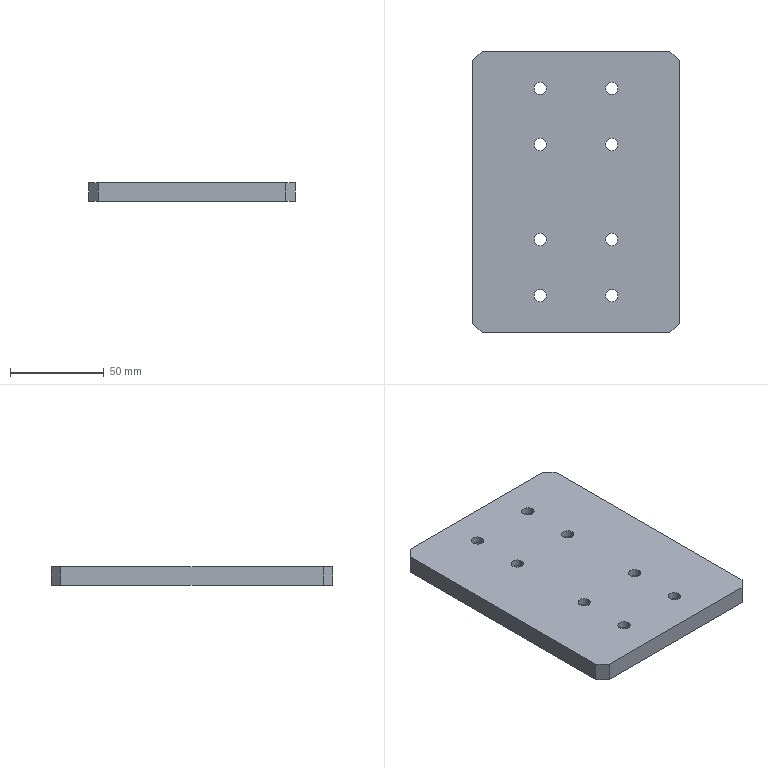Part | SolidWorks | features BaseBody 1 | 1 solid | 50 faces | box 110 x 150 x 10 mm | volume 158649 mm3 | cylinder 32 | plane 18 | commonest cylinder face diameters 6.6 x16 11 x16
STEP:
#1=CARTESIAN_POINT('',(-50.,75.,5.));
#2=VERTEX_POINT('',#1);
#3=CARTESIAN_POINT('',(-55.,70.,5.));
#4=VERTEX_POINT('',#3);
#5=CARTESIAN_POINT('',(-55.,70.,5.));
#6=DIRECTION('',(-0.7071,-0.7071,0.));
#7=VECTOR('',#6,1000.);
#8=LINE('',#5,#7);
#9=EDGE_CURVE('',#2,#4,#8,.T.);
#10=ORIENTED_EDGE('',*,*,#9,.F.);
#11=CARTESIAN_POINT('',(-50.,75.,-5.));
#12=VERTEX_POINT('',#11);
#13=CARTESIAN_POINT('',(-50.,75.,5.));
#14=DIRECTION('',(0.,0.,1.));
#15=VECTOR('',#14,1000.);
#16=LINE('',#13,#15);
#17=EDGE_CURVE('',#12,#2,#16,.T.);
#18=ORIENTED_EDGE('',*,*,#17,.F.);
#19=CARTESIAN_POINT('',(-55.,70.,-5.));
#20=VERTEX_POINT('',#19);
#21=CARTESIAN_POINT('',(-62.5,62.5,-5.));
#22=DIRECTION('',(0.7071,0.7071,0.));
#23=VECTOR('',#22,1000.);
#24=LINE('',#21,#23);
#25=EDGE_CURVE('',#20,#12,#24,.T.);
#26=ORIENTED_EDGE('',*,*,#25,.F.);
#27=CARTESIAN_POINT('',(-55.,70.,5.));
#28=DIRECTION('',(0.,0.,-1.));
#29=VECTOR('',#28,1000.);
#30=LINE('',#27,#29);
#31=EDGE_CURVE('',#4,#20,#30,.T.);
#32=ORIENTED_EDGE('',*,*,#31,.F.);
#33=EDGE_LOOP('',(#10,#18,#26,#32));
#34=FACE_OUTER_BOUND('',#33,.T.);
#35=CARTESIAN_POINT('',(-55.,70.,5.));
#36=DIRECTION('',(0.7071,-0.7071,0.));
#37=DIRECTION('',(0.,0.,-1.));
#38=AXIS2_PLACEMENT_3D('',#35,#36,#37);
#39=PLANE('',#38);
#40=ADVANCED_FACE('',(#34),#39,.F.);
#41=CARTESIAN_POINT('',(55.,70.,5.));
#42=VERTEX_POINT('',#41);
#43=CARTESIAN_POINT('',(50.,75.,5.));
#44=VERTEX_POINT('',#43);
#45=CARTESIAN_POINT('',(50.,75.,5.));
#46=DIRECTION('',(-0.7071,0.7071,0.));
#47=VECTOR('',#46,1000.);
#48=LINE('',#45,#47);
#49=EDGE_CURVE('',#42,#44,#48,.T.);
#50=ORIENTED_EDGE('',*,*,#49,.F.);
#51=CARTESIAN_POINT('',(55.,70.,-5.));
#52=VERTEX_POINT('',#51);
#53=CARTESIAN_POINT('',(55.,70.,5.));
#54=DIRECTION('',(0.,0.,1.));
#55=VECTOR('',#54,1000.);
#56=LINE('',#53,#55);
#57=EDGE_CURVE('',#52,#42,#56,.T.);
#58=ORIENTED_EDGE('',*,*,#57,.F.);
#59=CARTESIAN_POINT('',(50.,75.,-5.));
#60=VERTEX_POINT('',#59);
#61=CARTESIAN_POINT('',(62.5,62.5,-5.));
#62=DIRECTION('',(0.7071,-0.7071,0.));
#63=VECTOR('',#62,1000.);
#64=LINE('',#61,#63);
#65=EDGE_CURVE('',#60,#52,#64,.T.);
#66=ORIENTED_EDGE('',*,*,#65,.F.);
#67=CARTESIAN_POINT('',(50.,75.,5.));
#68=DIRECTION('',(0.,0.,-1.));
#69=VECTOR('',#68,1000.);
#70=LINE('',#67,#69);
#71=EDGE_CURVE('',#44,#60,#70,.T.);
#72=ORIENTED_EDGE('',*,*,#71,.F.);
#73=EDGE_LOOP('',(#50,#58,#66,#72));
#74=FACE_OUTER_BOUND('',#73,.T.);
#75=CARTESIAN_POINT('',(50.,75.,5.));
#76=DIRECTION('',(-0.7071,-0.7071,0.));
#77=DIRECTION('',(-0.7071,0.7071,0.));
#78=AXIS2_PLACEMENT_3D('',#75,#76,#77);
#79=PLANE('',#78);
#80=ADVANCED_FACE('',(#74),#79,.F.);
#81=CARTESIAN_POINT('',(-55.,-70.,5.));
#82=VERTEX_POINT('',#81);
#83=CARTESIAN_POINT('',(-50.,-75.,5.));
#84=VERTEX_POINT('',#83);
#85=CARTESIAN_POINT('',(-50.,-75.,5.));
#86=DIRECTION('',(0.7071,-0.7071,0.));
#87=VECTOR('',#86,1000.);
#88=LINE('',#85,#87);
#89=EDGE_CURVE('',#82,#84,#88,.T.);
#90=ORIENTED_EDGE('',*,*,#89,.F.);
#91=CARTESIAN_POINT('',(-55.,-70.,-5.));
#92=VERTEX_POINT('',#91);
#93=CARTESIAN_POINT('',(-55.,-70.,5.));
#94=DIRECTION('',(0.,0.,1.));
#95=VECTOR('',#94,1000.);
#96=LINE('',#93,#95);
#97=EDGE_CURVE('',#92,#82,#96,.T.);
#98=ORIENTED_EDGE('',*,*,#97,.F.);
#99=CARTESIAN_POINT('',(-50.,-75.,-5.));
#100=VERTEX_POINT('',#99);
#101=CARTESIAN_POINT('',(-62.5,-62.5,-5.));
#102=DIRECTION('',(-0.7071,0.7071,0.));
#103=VECTOR('',#102,1000.);
#104=LINE('',#101,#103);
#105=EDGE_CURVE('',#100,#92,#104,.T.);
#106=ORIENTED_EDGE('',*,*,#105,.F.);
#107=CARTESIAN_POINT('',(-50.,-75.,5.));
#108=DIRECTION('',(0.,0.,-1.));
#109=VECTOR('',#108,1000.);
#110=LINE('',#107,#109);
#111=EDGE_CURVE('',#84,#100,#110,.T.);
#112=ORIENTED_EDGE('',*,*,#111,.F.);
#113=EDGE_LOOP('',(#90,#98,#106,#112));
#114=FACE_OUTER_BOUND('',#113,.T.);
#115=CARTESIAN_POINT('',(-50.,-75.,5.));
#116=DIRECTION('',(0.7071,0.7071,0.));
#117=DIRECTION('',(0.,0.,-1.));
#118=AXIS2_PLACEMENT_3D('',#115,#116,#117);
#119=PLANE('',#118);
#120=ADVANCED_FACE('',(#114),#119,.F.);
#121=CARTESIAN_POINT('',(50.,-75.,5.));
#122=VERTEX_POINT('',#121);
#123=CARTESIAN_POINT('',(55.,-70.,5.));
#124=VERTEX_POINT('',#123);
#125=CARTESIAN_POINT('',(55.,-70.,5.));
#126=DIRECTION('',(0.7071,0.7071,0.));
#127=VECTOR('',#126,1000.);
#128=LINE('',#125,#127);
#129=EDGE_CURVE('',#122,#124,#128,.T.);
#130=ORIENTED_EDGE('',*,*,#129,.F.);
#131=CARTESIAN_POINT('',(50.,-75.,-5.));
#132=VERTEX_POINT('',#131);
#133=CARTESIAN_POINT('',(50.,-75.,5.));
#134=DIRECTION('',(0.,0.,1.));
#135=VECTOR('',#134,1000.);
#136=LINE('',#133,#135);
#137=EDGE_CURVE('',#132,#122,#136,.T.);
#138=ORIENTED_EDGE('',*,*,#137,.F.);
#139=CARTESIAN_POINT('',(55.,-70.,-5.));
#140=VERTEX_POINT('',#139);
#141=CARTESIAN_POINT('',(62.5,-62.5,-5.));
#142=DIRECTION('',(-0.7071,-0.7071,0.));
#143=VECTOR('',#142,1000.);
#144=LINE('',#141,#143);
#145=EDGE_CURVE('',#140,#132,#144,.T.);
#146=ORIENTED_EDGE('',*,*,#145,.F.);
#147=CARTESIAN_POINT('',(55.,-70.,5.));
#148=DIRECTION('',(0.,0.,-1.));
#149=VECTOR('',#148,1000.);
#150=LINE('',#147,#149);
#151=EDGE_CURVE('',#124,#140,#150,.T.);
#152=ORIENTED_EDGE('',*,*,#151,.F.);
#153=EDGE_LOOP('',(#130,#138,#146,#152));
#154=FACE_OUTER_BOUND('',#153,.T.);
#155=CARTESIAN_POINT('',(55.,-70.,5.));
#156=DIRECTION('',(-0.7071,0.7071,0.));
#157=DIRECTION('',(0.,0.,1.));
#158=AXIS2_PLACEMENT_3D('',#155,#156,#157);
#159=PLANE('',#158);
#160=ADVANCED_FACE('',(#154),#159,.F.);
#161=CARTESIAN_POINT('',(-13.5,-55.25,1.4));
#162=VERTEX_POINT('',#161);
#163=CARTESIAN_POINT('',(-13.5,-55.25,-5.));
#164=VERTEX_POINT('',#163);
#165=CARTESIAN_POINT('',(-13.5,-55.25,-5.));
#166=DIRECTION('',(0.,0.,-1.));
#167=VECTOR('',#166,1000.);
#168=LINE('',#165,#167);
#169=EDGE_CURVE('',#162,#164,#168,.T.);
#170=ORIENTED_EDGE('',*,*,#169,.F.);
#171=CARTESIAN_POINT('',(-24.5,-55.25,1.4));
#172=VERTEX_POINT('',#171);
#173=CARTESIAN_POINT('',(-19.,-55.25,1.4));
#174=DIRECTION('',(0.,0.,-1.));
#175=DIRECTION('',(-1.,0.,0.));
#176=AXIS2_PLACEMENT_3D('',#173,#174,#175);
#177=CIRCLE('',#176,5.5);
#178=EDGE_CURVE('',#172,#162,#177,.T.);
#179=ORIENTED_EDGE('',*,*,#178,.F.);
#180=CARTESIAN_POINT('',(-24.5,-55.25,-5.));
#181=VERTEX_POINT('',#180);
#182=CARTESIAN_POINT('',(-24.5,-55.25,-5.));
#183=DIRECTION('',(0.,0.,-1.));
#184=VECTOR('',#183,1000.);
#185=LINE('',#182,#184);
#186=EDGE_CURVE('',#172,#181,#185,.T.);
#187=ORIENTED_EDGE('',*,*,#186,.T.);
#188=CARTESIAN_POINT('',(-19.,-55.25,-5.));
#189=DIRECTION('',(0.,0.,-1.));
#190=DIRECTION('',(-1.,0.,0.));
#191=AXIS2_PLACEMENT_3D('',#188,#189,#190);
#192=CIRCLE('',#191,5.5);
#193=EDGE_CURVE('',#181,#164,#192,.T.);
#194=ORIENTED_EDGE('',*,*,#193,.T.);
#195=EDGE_LOOP('',(#170,#179,#187,#194));
#196=FACE_OUTER_BOUND('',#195,.T.);
#197=CARTESIAN_POINT('',(-19.,-55.25,-5.));
#198=DIRECTION('',(0.,0.,-1.));
#199=DIRECTION('',(-1.,0.,0.));
#200=AXIS2_PLACEMENT_3D('',#197,#198,#199);
#201=CYLINDRICAL_SURFACE('',#200,5.5);
#202=ADVANCED_FACE('',(#196),#201,.F.);
#203=CARTESIAN_POINT('',(-22.3,-55.25,1.4));
#204=VERTEX_POINT('',#203);
#205=CARTESIAN_POINT('',(-15.7,-55.25,1.4));
#206=VERTEX_POINT('',#205);
#207=CARTESIAN_POINT('',(-19.,-55.25,1.4));
#208=DIRECTION('',(0.,0.,-1.));
#209=DIRECTION('',(-1.,0.,0.));
#210=AXIS2_PLACEMENT_3D('',#207,#208,#209);
#211=CIRCLE('',#210,3.3);
#212=EDGE_CURVE('',#204,#206,#211,.T.);
#213=ORIENTED_EDGE('',*,*,#212,.F.);
#214=CARTESIAN_POINT('',(-19.,-55.25,1.4));
#215=DIRECTION('',(0.,0.,-1.));
#216=DIRECTION('',(-1.,0.,0.));
#217=AXIS2_PLACEMENT_3D('',#214,#215,#216);
#218=CIRCLE('',#217,3.3);
#219=EDGE_CURVE('',#206,#204,#218,.T.);
#220=ORIENTED_EDGE('',*,*,#219,.F.);
#221=EDGE_LOOP('',(#213,#220));
#222=FACE_BOUND('',#221,.T.);
#223=ORIENTED_EDGE('',*,*,#178,.T.);
#224=CARTESIAN_POINT('',(-19.,-55.25,1.4));
#225=DIRECTION('',(0.,0.,-1.));
#226=DIRECTION('',(-1.,0.,0.));
#227=AXIS2_PLACEMENT_3D('',#224,#225,#226);
#228=CIRCLE('',#227,5.5);
#229=EDGE_CURVE('',#162,#172,#228,.T.);
#230=ORIENTED_EDGE('',*,*,#229,.T.);
#231=EDGE_LOOP('',(#223,#230));
#232=FACE_OUTER_BOUND('',#231,.T.);
#233=CARTESIAN_POINT('',(-15.7,-55.25,1.4));
#234=DIRECTION('',(0.,0.,1.));
#235=DIRECTION('',(1.,0.,0.));
#236=AXIS2_PLACEMENT_3D('',#233,#234,#235);
#237=PLANE('',#236);
#238=ADVANCED_FACE('',(#222,#232),#237,.F.);
#239=CARTESIAN_POINT('',(-15.7,-55.25,5.));
#240=VERTEX_POINT('',#239);
#241=CARTESIAN_POINT('',(-15.7,-55.25,-5.));
#242=DIRECTION('',(0.,0.,-1.));
#243=VECTOR('',#242,1000.);
#244=LINE('',#241,#243);
#245=EDGE_CURVE('',#240,#206,#244,.T.);
#246=ORIENTED_EDGE('',*,*,#245,.F.);
#247=CARTESIAN_POINT('',(-22.3,-55.25,5.));
#248=VERTEX_POINT('',#247);
#249=CARTESIAN_POINT('',(-19.,-55.25,5.));
#250=DIRECTION('',(0.,0.,-1.));
#251=DIRECTION('',(-1.,0.,0.));
#252=AXIS2_PLACEMENT_3D('',#249,#250,#251);
#253=CIRCLE('',#252,3.3);
#254=EDGE_CURVE('',#248,#240,#253,.T.);
#255=ORIENTED_EDGE('',*,*,#254,.F.);
#256=CARTESIAN_POINT('',(-22.3,-55.25,-5.));
#257=DIRECTION('',(0.,0.,-1.));
#258=VECTOR('',#257,1000.);
#259=LINE('',#256,#258);
#260=EDGE_CURVE('',#248,#204,#259,.T.);
#261=ORIENTED_EDGE('',*,*,#260,.T.);
#262=ORIENTED_EDGE('',*,*,#212,.T.);
#263=EDGE_LOOP('',(#246,#255,#261,#262));
#264=FACE_OUTER_BOUND('',#263,.T.);
#265=CARTESIAN_POINT('',(-19.,-55.25,-5.));
#266=DIRECTION('',(0.,0.,-1.));
#267=DIRECTION('',(-1.,0.,0.));
#268=AXIS2_PLACEMENT_3D('',#265,#266,#267);
#269=CYLINDRICAL_SURFACE('',#268,3.3);
#270=ADVANCED_FACE('',(#264),#269,.F.);
#271=CARTESIAN_POINT('',(-13.5,25.25,1.4));
#272=VERTEX_POINT('',#271);
#273=CARTESIAN_POINT('',(-13.5,25.25,-5.));
#274=VERTEX_POINT('',#273);
#275=CARTESIAN_POINT('',(-13.5,25.25,-5.));
#276=DIRECTION('',(0.,0.,-1.));
#277=VECTOR('',#276,1000.);
#278=LINE('',#275,#277);
#279=EDGE_CURVE('',#272,#274,#278,.T.);
#280=ORIENTED_EDGE('',*,*,#279,.F.);
#281=CARTESIAN_POINT('',(-24.5,25.25,1.4));
#282=VERTEX_POINT('',#281);
#283=CARTESIAN_POINT('',(-19.,25.25,1.4));
#284=DIRECTION('',(0.,0.,-1.));
#285=DIRECTION('',(-1.,0.,0.));
#286=AXIS2_PLACEMENT_3D('',#283,#284,#285);
#287=CIRCLE('',#286,5.5);
#288=EDGE_CURVE('',#282,#272,#287,.T.);
#289=ORIENTED_EDGE('',*,*,#288,.F.);
#290=CARTESIAN_POINT('',(-24.5,25.25,-5.));
#291=VERTEX_POINT('',#290);
#292=CARTESIAN_POINT('',(-24.5,25.25,-5.));
#293=DIRECTION('',(0.,0.,-1.));
#294=VECTOR('',#293,1000.);
#295=LINE('',#292,#294);
#296=EDGE_CURVE('',#282,#291,#295,.T.);
#297=ORIENTED_EDGE('',*,*,#296,.T.);
#298=CARTESIAN_POINT('',(-19.,25.25,-5.));
#299=DIRECTION('',(0.,0.,-1.));
#300=DIRECTION('',(-1.,0.,0.));
#301=AXIS2_PLACEMENT_3D('',#298,#299,#300);
#302=CIRCLE('',#301,5.5);
#303=EDGE_CURVE('',#291,#274,#302,.T.);
#304=ORIENTED_EDGE('',*,*,#303,.T.);
#305=EDGE_LOOP('',(#280,#289,#297,#304));
#306=FACE_OUTER_BOUND('',#305,.T.);
#307=CARTESIAN_POINT('',(-19.,25.25,-5.));
#308=DIRECTION('',(0.,0.,-1.));
#309=DIRECTION('',(-1.,0.,0.));
#310=AXIS2_PLACEMENT_3D('',#307,#308,#309);
#311=CYLINDRICAL_SURFACE('',#310,5.5);
#312=ADVANCED_FACE('',(#306),#311,.F.);
#313=CARTESIAN_POINT('',(-22.3,25.25,1.4));
#314=VERTEX_POINT('',#313);
#315=CARTESIAN_POINT('',(-15.7,25.25,1.4));
#316=VERTEX_POINT('',#315);
#317=CARTESIAN_POINT('',(-19.,25.25,1.4));
#318=DIRECTION('',(0.,0.,-1.));
#319=DIRECTION('',(-1.,0.,0.));
#320=AXIS2_PLACEMENT_3D('',#317,#318,#319);
#321=CIRCLE('',#320,3.3);
#322=EDGE_CURVE('',#314,#316,#321,.T.);
#323=ORIENTED_EDGE('',*,*,#322,.F.);
#324=CARTESIAN_POINT('',(-19.,25.25,1.4));
#325=DIRECTION('',(0.,0.,-1.));
#326=DIRECTION('',(-1.,0.,0.));
#327=AXIS2_PLACEMENT_3D('',#324,#325,#326);
#328=CIRCLE('',#327,3.3);
#329=EDGE_CURVE('',#316,#314,#328,.T.);
#330=ORIENTED_EDGE('',*,*,#329,.F.);
#331=EDGE_LOOP('',(#323,#330));
#332=FACE_BOUND('',#331,.T.);
#333=ORIENTED_EDGE('',*,*,#288,.T.);
#334=CARTESIAN_POINT('',(-19.,25.25,1.4));
#335=DIRECTION('',(0.,0.,-1.));
#336=DIRECTION('',(-1.,0.,0.));
#337=AXIS2_PLACEMENT_3D('',#334,#335,#336);
#338=CIRCLE('',#337,5.5);
#339=EDGE_CURVE('',#272,#282,#338,.T.);
#340=ORIENTED_EDGE('',*,*,#339,.T.);
#341=EDGE_LOOP('',(#333,#340));
#342=FACE_OUTER_BOUND('',#341,.T.);
#343=CARTESIAN_POINT('',(-15.7,25.25,1.4));
#344=DIRECTION('',(0.,0.,1.));
#345=DIRECTION('',(1.,0.,0.));
#346=AXIS2_PLACEMENT_3D('',#343,#344,#345);
#347=PLANE('',#346);
#348=ADVANCED_FACE('',(#332,#342),#347,.F.);
#349=CARTESIAN_POINT('',(-15.7,25.25,5.));
#350=VERTEX_POINT('',#349);
#351=CARTESIAN_POINT('',(-15.7,25.25,-5.));
#352=DIRECTION('',(0.,0.,-1.));
#353=VECTOR('',#352,1000.);
#354=LINE('',#351,#353);
#355=EDGE_CURVE('',#350,#316,#354,.T.);
#356=ORIENTED_EDGE('',*,*,#355,.F.);
#357=CARTESIAN_POINT('',(-22.3,25.25,5.));
#358=VERTEX_POINT('',#357);
#359=CARTESIAN_POINT('',(-19.,25.25,5.));
#360=DIRECTION('',(0.,0.,-1.));
#361=DIRECTION('',(-1.,0.,0.));
#362=AXIS2_PLACEMENT_3D('',#359,#360,#361);
#363=CIRCLE('',#362,3.3);
#364=EDGE_CURVE('',#358,#350,#363,.T.);
#365=ORIENTED_EDGE('',*,*,#364,.F.);
#366=CARTESIAN_POINT('',(-22.3,25.25,-5.));
#367=DIRECTION('',(0.,0.,-1.));
#368=VECTOR('',#367,1000.);
#369=LINE('',#366,#368);
#370=EDGE_CURVE('',#358,#314,#369,.T.);
#371=ORIENTED_EDGE('',*,*,#370,.T.);
#372=ORIENTED_EDGE('',*,*,#322,.T.);
#373=EDGE_LOOP('',(#356,#365,#371,#372));
#374=FACE_OUTER_BOUND('',#373,.T.);
#375=CARTESIAN_POINT('',(-19.,25.25,-5.));
#376=DIRECTION('',(0.,0.,-1.));
#377=DIRECTION('',(-1.,0.,0.));
#378=AXIS2_PLACEMENT_3D('',#375,#376,#377);
#379=CYLINDRICAL_SURFACE('',#378,3.3);
#380=ADVANCED_FACE('',(#374),#379,.F.);
#381=CARTESIAN_POINT('',(-13.5,55.25,1.4));
#382=VERTEX_POINT('',#381);
#383=CARTESIAN_POINT('',(-13.5,55.25,-5.));
#384=VERTEX_POINT('',#383);
#385=CARTESIAN_POINT('',(-13.5,55.25,-5.));
#386=DIRECTION('',(0.,0.,-1.));
#387=VECTOR('',#386,1000.);
#388=LINE('',#385,#387);
#389=EDGE_CURVE('',#382,#384,#388,.T.);
#390=ORIENTED_EDGE('',*,*,#389,.F.);
#391=CARTESIAN_POINT('',(-24.5,55.25,1.4));
#392=VERTEX_POINT('',#391);
#393=CARTESIAN_POINT('',(-19.,55.25,1.4));
#394=DIRECTION('',(0.,0.,-1.));
#395=DIRECTION('',(-1.,0.,0.));
#396=AXIS2_PLACEMENT_3D('',#393,#394,#395);
#397=CIRCLE('',#396,5.5);
#398=EDGE_CURVE('',#392,#382,#397,.T.);
#399=ORIENTED_EDGE('',*,*,#398,.F.);
#400=CARTESIAN_POINT('',(-24.5,55.25,-5.));
#401=VERTEX_POINT('',#400);
#402=CARTESIAN_POINT('',(-24.5,55.25,-5.));
#403=DIRECTION('',(0.,0.,-1.));
#404=VECTOR('',#403,1000.);
#405=LINE('',#402,#404);
#406=EDGE_CURVE('',#392,#401,#405,.T.);
#407=ORIENTED_EDGE('',*,*,#406,.T.);
#408=CARTESIAN_POINT('',(-19.,55.25,-5.));
#409=DIRECTION('',(0.,0.,-1.));
#410=DIRECTION('',(-1.,0.,0.));
#411=AXIS2_PLACEMENT_3D('',#408,#409,#410);
#412=CIRCLE('',#411,5.5);
#413=EDGE_CURVE('',#401,#384,#412,.T.);
#414=ORIENTED_EDGE('',*,*,#413,.T.);
#415=EDGE_LOOP('',(#390,#399,#407,#414));
#416=FACE_OUTER_BOUND('',#415,.T.);
#417=CARTESIAN_POINT('',(-19.,55.25,-5.));
#418=DIRECTION('',(0.,0.,-1.));
#419=DIRECTION('',(-1.,0.,0.));
#420=AXIS2_PLACEMENT_3D('',#417,#418,#419);
#421=CYLINDRICAL_SURFACE('',#420,5.5);
#422=ADVANCED_FACE('',(#416),#421,.F.);
#423=CARTESIAN_POINT('',(-22.3,55.25,1.4));
#424=VERTEX_POINT('',#423);
#425=CARTESIAN_POINT('',(-15.7,55.25,1.4));
#426=VERTEX_POINT('',#425);
#427=CARTESIAN_POINT('',(-19.,55.25,1.4));
#428=DIRECTION('',(0.,0.,-1.));
#429=DIRECTION('',(-1.,0.,0.));
#430=AXIS2_PLACEMENT_3D('',#427,#428,#429);
#431=CIRCLE('',#430,3.3);
#432=EDGE_CURVE('',#424,#426,#431,.T.);
#433=ORIENTED_EDGE('',*,*,#432,.F.);
#434=CARTESIAN_POINT('',(-19.,55.25,1.4));
#435=DIRECTION('',(0.,0.,-1.));
#436=DIRECTION('',(-1.,0.,0.));
#437=AXIS2_PLACEMENT_3D('',#434,#435,#436);
#438=CIRCLE('',#437,3.3);
#439=EDGE_CURVE('',#426,#424,#438,.T.);
#440=ORIENTED_EDGE('',*,*,#439,.F.);
#441=EDGE_LOOP('',(#433,#440));
#442=FACE_BOUND('',#441,.T.);
#443=ORIENTED_EDGE('',*,*,#398,.T.);
#444=CARTESIAN_POINT('',(-19.,55.25,1.4));
#445=DIRECTION('',(0.,0.,-1.));
#446=DIRECTION('',(-1.,0.,0.));
#447=AXIS2_PLACEMENT_3D('',#444,#445,#446);
#448=CIRCLE('',#447,5.5);
#449=EDGE_CURVE('',#382,#392,#448,.T.);
#450=ORIENTED_EDGE('',*,*,#449,.T.);
#451=EDGE_LOOP('',(#443,#450));
#452=FACE_OUTER_BOUND('',#451,.T.);
#453=CARTESIAN_POINT('',(-15.7,55.25,1.4));
#454=DIRECTION('',(0.,0.,1.));
#455=DIRECTION('',(1.,0.,0.));
#456=AXIS2_PLACEMENT_3D('',#453,#454,#455);
#457=PLANE('',#456);
#458=ADVANCED_FACE('',(#442,#452),#457,.F.);
#459=CARTESIAN_POINT('',(-15.7,55.25,5.));
#460=VERTEX_POINT('',#459);
#461=CARTESIAN_POINT('',(-15.7,55.25,-5.));
#462=DIRECTION('',(0.,0.,-1.));
#463=VECTOR('',#462,1000.);
#464=LINE('',#461,#463);
#465=EDGE_CURVE('',#460,#426,#464,.T.);
#466=ORIENTED_EDGE('',*,*,#465,.F.);
#467=CARTESIAN_POINT('',(-22.3,55.25,5.));
#468=VERTEX_POINT('',#467);
#469=CARTESIAN_POINT('',(-19.,55.25,5.));
#470=DIRECTION('',(0.,0.,-1.));
#471=DIRECTION('',(-1.,0.,0.));
#472=AXIS2_PLACEMENT_3D('',#469,#470,#471);
#473=CIRCLE('',#472,3.3);
#474=EDGE_CURVE('',#468,#460,#473,.T.);
#475=ORIENTED_EDGE('',*,*,#474,.F.);
#476=CARTESIAN_POINT('',(-22.3,55.25,-5.));
#477=DIRECTION('',(0.,0.,-1.));
#478=VECTOR('',#477,1000.);
#479=LINE('',#476,#478);
#480=EDGE_CURVE('',#468,#424,#479,.T.);
#481=ORIENTED_EDGE('',*,*,#480,.T.);
#482=ORIENTED_EDGE('',*,*,#432,.T.);
#483=EDGE_LOOP('',(#466,#475,#481,#482));
#484=FACE_OUTER_BOUND('',#483,.T.);
#485=CARTESIAN_POINT('',(-19.,55.25,-5.));
#486=DIRECTION('',(0.,0.,-1.));
#487=DIRECTION('',(-1.,0.,0.));
#488=AXIS2_PLACEMENT_3D('',#485,#486,#487);
#489=CYLINDRICAL_SURFACE('',#488,3.3);
#490=ADVANCED_FACE('',(#484),#489,.F.);
#491=CARTESIAN_POINT('',(-13.5,-25.25,1.4));
#492=VERTEX_POINT('',#491);
#493=CARTESIAN_POINT('',(-13.5,-25.25,-5.));
#494=VERTEX_POINT('',#493);
#495=CARTESIAN_POINT('',(-13.5,-25.25,-5.));
#496=DIRECTION('',(0.,0.,-1.));
#497=VECTOR('',#496,1000.);
#498=LINE('',#495,#497);
#499=EDGE_CURVE('',#492,#494,#498,.T.);
#500=ORIENTED_EDGE('',*,*,#499,.F.);
#501=CARTESIAN_POINT('',(-24.5,-25.25,1.4));
#502=VERTEX_POINT('',#501);
#503=CARTESIAN_POINT('',(-19.,-25.25,1.4));
#504=DIRECTION('',(0.,0.,-1.));
#505=DIRECTION('',(-1.,0.,0.));
#506=AXIS2_PLACEMENT_3D('',#503,#504,#505);
#507=CIRCLE('',#506,5.5);
#508=EDGE_CURVE('',#502,#492,#507,.T.);
#509=ORIENTED_EDGE('',*,*,#508,.F.);
#510=CARTESIAN_POINT('',(-24.5,-25.25,-5.));
#511=VERTEX_POINT('',#510);
#512=CARTESIAN_POINT('',(-24.5,-25.25,-5.));
#513=DIRECTION('',(0.,0.,-1.));
#514=VECTOR('',#513,1000.);
#515=LINE('',#512,#514);
#516=EDGE_CURVE('',#502,#511,#515,.T.);
#517=ORIENTED_EDGE('',*,*,#516,.T.);
#518=CARTESIAN_POINT('',(-19.,-25.25,-5.));
#519=DIRECTION('',(0.,0.,-1.));
#520=DIRECTION('',(-1.,0.,0.));
#521=AXIS2_PLACEMENT_3D('',#518,#519,#520);
#522=CIRCLE('',#521,5.5);
#523=EDGE_CURVE('',#511,#494,#522,.T.);
#524=ORIENTED_EDGE('',*,*,#523,.T.);
#525=EDGE_LOOP('',(#500,#509,#517,#524));
#526=FACE_OUTER_BOUND('',#525,.T.);
#527=CARTESIAN_POINT('',(-19.,-25.25,-5.));
#528=DIRECTION('',(0.,0.,-1.));
#529=DIRECTION('',(-1.,0.,0.));
#530=AXIS2_PLACEMENT_3D('',#527,#528,#529);
#531=CYLINDRICAL_SURFACE('',#530,5.5);
#532=ADVANCED_FACE('',(#526),#531,.F.);
#533=CARTESIAN_POINT('',(-22.3,-25.25,1.4));
#534=VERTEX_POINT('',#533);
#535=CARTESIAN_POINT('',(-15.7,-25.25,1.4));
#536=VERTEX_POINT('',#535);
#537=CARTESIAN_POINT('',(-19.,-25.25,1.4));
#538=DIRECTION('',(0.,0.,-1.));
#539=DIRECTION('',(-1.,0.,0.));
#540=AXIS2_PLACEMENT_3D('',#537,#538,#539);
#541=CIRCLE('',#540,3.3);
#542=EDGE_CURVE('',#534,#536,#541,.T.);
#543=ORIENTED_EDGE('',*,*,#542,.F.);
#544=CARTESIAN_POINT('',(-19.,-25.25,1.4));
#545=DIRECTION('',(0.,0.,-1.));
#546=DIRECTION('',(-1.,0.,0.));
#547=AXIS2_PLACEMENT_3D('',#544,#545,#546);
#548=CIRCLE('',#547,3.3);
#549=EDGE_CURVE('',#536,#534,#548,.T.);
#550=ORIENTED_EDGE('',*,*,#549,.F.);
#551=EDGE_LOOP('',(#543,#550));
#552=FACE_BOUND('',#551,.T.);
#553=ORIENTED_EDGE('',*,*,#508,.T.);
#554=CARTESIAN_POINT('',(-19.,-25.25,1.4));
#555=DIRECTION('',(0.,0.,-1.));
#556=DIRECTION('',(-1.,0.,0.));
#557=AXIS2_PLACEMENT_3D('',#554,#555,#556);
#558=CIRCLE('',#557,5.5);
#559=EDGE_CURVE('',#492,#502,#558,.T.);
#560=ORIENTED_EDGE('',*,*,#559,.T.);
#561=EDGE_LOOP('',(#553,#560));
#562=FACE_OUTER_BOUND('',#561,.T.);
#563=CARTESIAN_POINT('',(-15.7,-25.25,1.4));
#564=DIRECTION('',(0.,0.,1.));
#565=DIRECTION('',(1.,0.,0.));
#566=AXIS2_PLACEMENT_3D('',#563,#564,#565);
#567=PLANE('',#566);
#568=ADVANCED_FACE('',(#552,#562),#567,.F.);
#569=CARTESIAN_POINT('',(-15.7,-25.25,5.));
#570=VERTEX_POINT('',#569);
#571=CARTESIAN_POINT('',(-15.7,-25.25,-5.));
#572=DIRECTION('',(0.,0.,-1.));
#573=VECTOR('',#572,1000.);
#574=LINE('',#571,#573);
#575=EDGE_CURVE('',#570,#536,#574,.T.);
#576=ORIENTED_EDGE('',*,*,#575,.F.);
#577=CARTESIAN_POINT('',(-22.3,-25.25,5.));
#578=VERTEX_POINT('',#577);
#579=CARTESIAN_POINT('',(-19.,-25.25,5.));
#580=DIRECTION('',(0.,0.,-1.));
#581=DIRECTION('',(-1.,0.,0.));
#582=AXIS2_PLACEMENT_3D('',#579,#580,#581);
#583=CIRCLE('',#582,3.3);
#584=EDGE_CURVE('',#578,#570,#583,.T.);
#585=ORIENTED_EDGE('',*,*,#584,.F.);
#586=CARTESIAN_POINT('',(-22.3,-25.25,-5.));
#587=DIRECTION('',(0.,0.,-1.));
#588=VECTOR('',#587,1000.);
#589=LINE('',#586,#588);
#590=EDGE_CURVE('',#578,#534,#589,.T.);
#591=ORIENTED_EDGE('',*,*,#590,.T.);
#592=ORIENTED_EDGE('',*,*,#542,.T.);
#593=EDGE_LOOP('',(#576,#585,#591,#592));
#594=FACE_OUTER_BOUND('',#593,.T.);
#595=CARTESIAN_POINT('',(-19.,-25.25,-5.));
#596=DIRECTION('',(0.,0.,-1.));
#597=DIRECTION('',(-1.,0.,0.));
#598=AXIS2_PLACEMENT_3D('',#595,#596,#597);
#599=CYLINDRICAL_SURFACE('',#598,3.3);
#600=ADVANCED_FACE('',(#594),#599,.F.);
#601=CARTESIAN_POINT('',(24.5,-55.25,1.4));
#602=VERTEX_POINT('',#601);
#603=CARTESIAN_POINT('',(24.5,-55.25,-5.));
#604=VERTEX_POINT('',#603);
#605=CARTESIAN_POINT('',(24.5,-55.25,-5.));
#606=DIRECTION('',(0.,0.,-1.));
#607=VECTOR('',#606,1000.);
#608=LINE('',#605,#607);
#609=EDGE_CURVE('',#602,#604,#608,.T.);
#610=ORIENTED_EDGE('',*,*,#609,.F.);
#611=CARTESIAN_POINT('',(13.5,-55.25,1.4));
#612=VERTEX_POINT('',#611);
#613=CARTESIAN_POINT('',(19.,-55.25,1.4));
#614=DIRECTION('',(0.,0.,-1.));
#615=DIRECTION('',(-1.,0.,0.));
#616=AXIS2_PLACEMENT_3D('',#613,#614,#615);
#617=CIRCLE('',#616,5.5);
#618=EDGE_CURVE('',#612,#602,#617,.T.);
#619=ORIENTED_EDGE('',*,*,#618,.F.);
#620=CARTESIAN_POINT('',(13.5,-55.25,-5.));
#621=VERTEX_POINT('',#620);
#622=CARTESIAN_POINT('',(13.5,-55.25,-5.));
#623=DIRECTION('',(0.,0.,-1.));
#624=VECTOR('',#623,1000.);
#625=LINE('',#622,#624);
#626=EDGE_CURVE('',#612,#621,#625,.T.);
#627=ORIENTED_EDGE('',*,*,#626,.T.);
#628=CARTESIAN_POINT('',(19.,-55.25,-5.));
#629=DIRECTION('',(0.,0.,-1.));
#630=DIRECTION('',(-1.,0.,0.));
#631=AXIS2_PLACEMENT_3D('',#628,#629,#630);
#632=CIRCLE('',#631,5.5);
#633=EDGE_CURVE('',#621,#604,#632,.T.);
#634=ORIENTED_EDGE('',*,*,#633,.T.);
#635=EDGE_LOOP('',(#610,#619,#627,#634));
#636=FACE_OUTER_BOUND('',#635,.T.);
#637=CARTESIAN_POINT('',(19.,-55.25,-5.));
#638=DIRECTION('',(0.,0.,-1.));
#639=DIRECTION('',(-1.,0.,0.));
#640=AXIS2_PLACEMENT_3D('',#637,#638,#639);
#641=CYLINDRICAL_SURFACE('',#640,5.5);
#642=ADVANCED_FACE('',(#636),#641,.F.);
#643=CARTESIAN_POINT('',(15.7,-55.25,1.4));
#644=VERTEX_POINT('',#643);
#645=CARTESIAN_POINT('',(22.3,-55.25,1.4));
#646=VERTEX_POINT('',#645);
#647=CARTESIAN_POINT('',(19.,-55.25,1.4));
#648=DIRECTION('',(0.,0.,-1.));
#649=DIRECTION('',(-1.,0.,0.));
#650=AXIS2_PLACEMENT_3D('',#647,#648,#649);
#651=CIRCLE('',#650,3.3);
#652=EDGE_CURVE('',#644,#646,#651,.T.);
#653=ORIENTED_EDGE('',*,*,#652,.F.);
#654=CARTESIAN_POINT('',(19.,-55.25,1.4));
#655=DIRECTION('',(0.,0.,-1.));
#656=DIRECTION('',(-1.,0.,0.));
#657=AXIS2_PLACEMENT_3D('',#654,#655,#656);
#658=CIRCLE('',#657,3.3);
#659=EDGE_CURVE('',#646,#644,#658,.T.);
#660=ORIENTED_EDGE('',*,*,#659,.F.);
#661=EDGE_LOOP('',(#653,#660));
#662=FACE_BOUND('',#661,.T.);
#663=ORIENTED_EDGE('',*,*,#618,.T.);
#664=CARTESIAN_POINT('',(19.,-55.25,1.4));
#665=DIRECTION('',(0.,0.,-1.));
#666=DIRECTION('',(-1.,0.,0.));
#667=AXIS2_PLACEMENT_3D('',#664,#665,#666);
#668=CIRCLE('',#667,5.5);
#669=EDGE_CURVE('',#602,#612,#668,.T.);
#670=ORIENTED_EDGE('',*,*,#669,.T.);
#671=EDGE_LOOP('',(#663,#670));
#672=FACE_OUTER_BOUND('',#671,.T.);
#673=CARTESIAN_POINT('',(22.3,-55.25,1.4));
#674=DIRECTION('',(0.,0.,1.));
#675=DIRECTION('',(1.,0.,0.));
#676=AXIS2_PLACEMENT_3D('',#673,#674,#675);
#677=PLANE('',#676);
#678=ADVANCED_FACE('',(#662,#672),#677,.F.);
#679=CARTESIAN_POINT('',(22.3,-55.25,5.));
#680=VERTEX_POINT('',#679);
#681=CARTESIAN_POINT('',(22.3,-55.25,-5.));
#682=DIRECTION('',(0.,0.,-1.));
#683=VECTOR('',#682,1000.);
#684=LINE('',#681,#683);
#685=EDGE_CURVE('',#680,#646,#684,.T.);
#686=ORIENTED_EDGE('',*,*,#685,.F.);
#687=CARTESIAN_POINT('',(15.7,-55.25,5.));
#688=VERTEX_POINT('',#687);
#689=CARTESIAN_POINT('',(19.,-55.25,5.));
#690=DIRECTION('',(0.,0.,-1.));
#691=DIRECTION('',(-1.,0.,0.));
#692=AXIS2_PLACEMENT_3D('',#689,#690,#691);
#693=CIRCLE('',#692,3.3);
#694=EDGE_CURVE('',#688,#680,#693,.T.);
#695=ORIENTED_EDGE('',*,*,#694,.F.);
#696=CARTESIAN_POINT('',(15.7,-55.25,-5.));
#697=DIRECTION('',(0.,0.,-1.));
#698=VECTOR('',#697,1000.);
#699=LINE('',#696,#698);
#700=EDGE_CURVE('',#688,#644,#699,.T.);
#701=ORIENTED_EDGE('',*,*,#700,.T.);
#702=ORIENTED_EDGE('',*,*,#652,.T.);
#703=EDGE_LOOP('',(#686,#695,#701,#702));
#704=FACE_OUTER_BOUND('',#703,.T.);
#705=CARTESIAN_POINT('',(19.,-55.25,-5.));
#706=DIRECTION('',(0.,0.,-1.));
#707=DIRECTION('',(-1.,0.,0.));
#708=AXIS2_PLACEMENT_3D('',#705,#706,#707);
#709=CYLINDRICAL_SURFACE('',#708,3.3);
#710=ADVANCED_FACE('',(#704),#709,.F.);
#711=CARTESIAN_POINT('',(24.5,-25.25,1.4));
#712=VERTEX_POINT('',#711);
#713=CARTESIAN_POINT('',(24.5,-25.25,-5.));
#714=VERTEX_POINT('',#713);
#715=CARTESIAN_POINT('',(24.5,-25.25,-5.));
#716=DIRECTION('',(0.,0.,-1.));
#717=VECTOR('',#716,1000.);
#718=LINE('',#715,#717);
#719=EDGE_CURVE('',#712,#714,#718,.T.);
#720=ORIENTED_EDGE('',*,*,#719,.F.);
#721=CARTESIAN_POINT('',(13.5,-25.25,1.4));
#722=VERTEX_POINT('',#721);
#723=CARTESIAN_POINT('',(19.,-25.25,1.4));
#724=DIRECTION('',(0.,0.,-1.));
#725=DIRECTION('',(-1.,0.,0.));
#726=AXIS2_PLACEMENT_3D('',#723,#724,#725);
#727=CIRCLE('',#726,5.5);
#728=EDGE_CURVE('',#722,#712,#727,.T.);
#729=ORIENTED_EDGE('',*,*,#728,.F.);
#730=CARTESIAN_POINT('',(13.5,-25.25,-5.));
#731=VERTEX_POINT('',#730);
#732=CARTESIAN_POINT('',(13.5,-25.25,-5.));
#733=DIRECTION('',(0.,0.,-1.));
#734=VECTOR('',#733,1000.);
#735=LINE('',#732,#734);
#736=EDGE_CURVE('',#722,#731,#735,.T.);
#737=ORIENTED_EDGE('',*,*,#736,.T.);
#738=CARTESIAN_POINT('',(19.,-25.25,-5.));
#739=DIRECTION('',(0.,0.,-1.));
#740=DIRECTION('',(-1.,0.,0.));
#741=AXIS2_PLACEMENT_3D('',#738,#739,#740);
#742=CIRCLE('',#741,5.5);
#743=EDGE_CURVE('',#731,#714,#742,.T.);
#744=ORIENTED_EDGE('',*,*,#743,.T.);
#745=EDGE_LOOP('',(#720,#729,#737,#744));
#746=FACE_OUTER_BOUND('',#745,.T.);
#747=CARTESIAN_POINT('',(19.,-25.25,-5.));
#748=DIRECTION('',(0.,0.,-1.));
#749=DIRECTION('',(-1.,0.,0.));
#750=AXIS2_PLACEMENT_3D('',#747,#748,#749);
#751=CYLINDRICAL_SURFACE('',#750,5.5);
#752=ADVANCED_FACE('',(#746),#751,.F.);
#753=CARTESIAN_POINT('',(15.7,-25.25,1.4));
#754=VERTEX_POINT('',#753);
#755=CARTESIAN_POINT('',(22.3,-25.25,1.4));
#756=VERTEX_POINT('',#755);
#757=CARTESIAN_POINT('',(19.,-25.25,1.4));
#758=DIRECTION('',(0.,0.,-1.));
#759=DIRECTION('',(-1.,0.,0.));
#760=AXIS2_PLACEMENT_3D('',#757,#758,#759);
#761=CIRCLE('',#760,3.3);
#762=EDGE_CURVE('',#754,#756,#761,.T.);
#763=ORIENTED_EDGE('',*,*,#762,.F.);
#764=CARTESIAN_POINT('',(19.,-25.25,1.4));
#765=DIRECTION('',(0.,0.,-1.));
#766=DIRECTION('',(-1.,0.,0.));
#767=AXIS2_PLACEMENT_3D('',#764,#765,#766);
#768=CIRCLE('',#767,3.3);
#769=EDGE_CURVE('',#756,#754,#768,.T.);
#770=ORIENTED_EDGE('',*,*,#769,.F.);
#771=EDGE_LOOP('',(#763,#770));
#772=FACE_BOUND('',#771,.T.);
#773=ORIENTED_EDGE('',*,*,#728,.T.);
#774=CARTESIAN_POINT('',(19.,-25.25,1.4));
#775=DIRECTION('',(0.,0.,-1.));
#776=DIRECTION('',(-1.,0.,0.));
#777=AXIS2_PLACEMENT_3D('',#774,#775,#776);
#778=CIRCLE('',#777,5.5);
#779=EDGE_CURVE('',#712,#722,#778,.T.);
#780=ORIENTED_EDGE('',*,*,#779,.T.);
#781=EDGE_LOOP('',(#773,#780));
#782=FACE_OUTER_BOUND('',#781,.T.);
#783=CARTESIAN_POINT('',(22.3,-25.25,1.4));
#784=DIRECTION('',(0.,0.,1.));
#785=DIRECTION('',(1.,0.,0.));
#786=AXIS2_PLACEMENT_3D('',#783,#784,#785);
#787=PLANE('',#786);
#788=ADVANCED_FACE('',(#772,#782),#787,.F.);
#789=CARTESIAN_POINT('',(22.3,-25.25,5.));
#790=VERTEX_POINT('',#789);
#791=CARTESIAN_POINT('',(22.3,-25.25,-5.));
#792=DIRECTION('',(0.,0.,-1.));
#793=VECTOR('',#792,1000.);
#794=LINE('',#791,#793);
#795=EDGE_CURVE('',#790,#756,#794,.T.);
#796=ORIENTED_EDGE('',*,*,#795,.F.);
#797=CARTESIAN_POINT('',(15.7,-25.25,5.));
#798=VERTEX_POINT('',#797);
#799=CARTESIAN_POINT('',(19.,-25.25,5.));
#800=DIRECTION('',(0.,0.,-1.));
#801=DIRECTION('',(-1.,0.,0.));
#802=AXIS2_PLACEMENT_3D('',#799,#800,#801);
#803=CIRCLE('',#802,3.3);
#804=EDGE_CURVE('',#798,#790,#803,.T.);
#805=ORIENTED_EDGE('',*,*,#804,.F.);
#806=CARTESIAN_POINT('',(15.7,-25.25,-5.));
#807=DIRECTION('',(0.,0.,-1.));
#808=VECTOR('',#807,1000.);
#809=LINE('',#806,#808);
#810=EDGE_CURVE('',#798,#754,#809,.T.);
#811=ORIENTED_EDGE('',*,*,#810,.T.);
#812=ORIENTED_EDGE('',*,*,#762,.T.);
#813=EDGE_LOOP('',(#796,#805,#811,#812));
#814=FACE_OUTER_BOUND('',#813,.T.);
#815=CARTESIAN_POINT('',(19.,-25.25,-5.));
#816=DIRECTION('',(0.,0.,-1.));
#817=DIRECTION('',(-1.,0.,0.));
#818=AXIS2_PLACEMENT_3D('',#815,#816,#817);
#819=CYLINDRICAL_SURFACE('',#818,3.3);
#820=ADVANCED_FACE('',(#814),#819,.F.);
#821=CARTESIAN_POINT('',(24.5,25.25,1.4));
#822=VERTEX_POINT('',#821);
#823=CARTESIAN_POINT('',(24.5,25.25,-5.));
#824=VERTEX_POINT('',#823);
#825=CARTESIAN_POINT('',(24.5,25.25,-5.));
#826=DIRECTION('',(0.,0.,-1.));
#827=VECTOR('',#826,1000.);
#828=LINE('',#825,#827);
#829=EDGE_CURVE('',#822,#824,#828,.T.);
#830=ORIENTED_EDGE('',*,*,#829,.F.);
#831=CARTESIAN_POINT('',(13.5,25.25,1.4));
#832=VERTEX_POINT('',#831);
#833=CARTESIAN_POINT('',(19.,25.25,1.4));
#834=DIRECTION('',(0.,0.,-1.));
#835=DIRECTION('',(-1.,0.,0.));
#836=AXIS2_PLACEMENT_3D('',#833,#834,#835);
#837=CIRCLE('',#836,5.5);
#838=EDGE_CURVE('',#832,#822,#837,.T.);
#839=ORIENTED_EDGE('',*,*,#838,.F.);
#840=CARTESIAN_POINT('',(13.5,25.25,-5.));
#841=VERTEX_POINT('',#840);
#842=CARTESIAN_POINT('',(13.5,25.25,-5.));
#843=DIRECTION('',(0.,0.,-1.));
#844=VECTOR('',#843,1000.);
#845=LINE('',#842,#844);
#846=EDGE_CURVE('',#832,#841,#845,.T.);
#847=ORIENTED_EDGE('',*,*,#846,.T.);
#848=CARTESIAN_POINT('',(19.,25.25,-5.));
#849=DIRECTION('',(0.,0.,-1.));
#850=DIRECTION('',(-1.,0.,0.));
#851=AXIS2_PLACEMENT_3D('',#848,#849,#850);
#852=CIRCLE('',#851,5.5);
#853=EDGE_CURVE('',#841,#824,#852,.T.);
#854=ORIENTED_EDGE('',*,*,#853,.T.);
#855=EDGE_LOOP('',(#830,#839,#847,#854));
#856=FACE_OUTER_BOUND('',#855,.T.);
#857=CARTESIAN_POINT('',(19.,25.25,-5.));
#858=DIRECTION('',(0.,0.,-1.));
#859=DIRECTION('',(-1.,0.,0.));
#860=AXIS2_PLACEMENT_3D('',#857,#858,#859);
#861=CYLINDRICAL_SURFACE('',#860,5.5);
#862=ADVANCED_FACE('',(#856),#861,.F.);
#863=CARTESIAN_POINT('',(15.7,25.25,1.4));
#864=VERTEX_POINT('',#863);
#865=CARTESIAN_POINT('',(22.3,25.25,1.4));
#866=VERTEX_POINT('',#865);
#867=CARTESIAN_POINT('',(19.,25.25,1.4));
#868=DIRECTION('',(0.,0.,-1.));
#869=DIRECTION('',(-1.,0.,0.));
#870=AXIS2_PLACEMENT_3D('',#867,#868,#869);
#871=CIRCLE('',#870,3.3);
#872=EDGE_CURVE('',#864,#866,#871,.T.);
#873=ORIENTED_EDGE('',*,*,#872,.F.);
#874=CARTESIAN_POINT('',(19.,25.25,1.4));
#875=DIRECTION('',(0.,0.,-1.));
#876=DIRECTION('',(-1.,0.,0.));
#877=AXIS2_PLACEMENT_3D('',#874,#875,#876);
#878=CIRCLE('',#877,3.3);
#879=EDGE_CURVE('',#866,#864,#878,.T.);
#880=ORIENTED_EDGE('',*,*,#879,.F.);
#881=EDGE_LOOP('',(#873,#880));
#882=FACE_BOUND('',#881,.T.);
#883=ORIENTED_EDGE('',*,*,#838,.T.);
#884=CARTESIAN_POINT('',(19.,25.25,1.4));
#885=DIRECTION('',(0.,0.,-1.));
#886=DIRECTION('',(-1.,0.,0.));
#887=AXIS2_PLACEMENT_3D('',#884,#885,#886);
#888=CIRCLE('',#887,5.5);
#889=EDGE_CURVE('',#822,#832,#888,.T.);
#890=ORIENTED_EDGE('',*,*,#889,.T.);
#891=EDGE_LOOP('',(#883,#890));
#892=FACE_OUTER_BOUND('',#891,.T.);
#893=CARTESIAN_POINT('',(22.3,25.25,1.4));
#894=DIRECTION('',(0.,0.,1.));
#895=DIRECTION('',(1.,0.,0.));
#896=AXIS2_PLACEMENT_3D('',#893,#894,#895);
#897=PLANE('',#896);
#898=ADVANCED_FACE('',(#882,#892),#897,.F.);
#899=CARTESIAN_POINT('',(22.3,25.25,5.));
#900=VERTEX_POINT('',#899);
#901=CARTESIAN_POINT('',(22.3,25.25,-5.));
#902=DIRECTION('',(0.,0.,-1.));
#903=VECTOR('',#902,1000.);
#904=LINE('',#901,#903);
#905=EDGE_CURVE('',#900,#866,#904,.T.);
#906=ORIENTED_EDGE('',*,*,#905,.F.);
#907=CARTESIAN_POINT('',(15.7,25.25,5.));
#908=VERTEX_POINT('',#907);
#909=CARTESIAN_POINT('',(19.,25.25,5.));
#910=DIRECTION('',(0.,0.,-1.));
#911=DIRECTION('',(-1.,0.,0.));
#912=AXIS2_PLACEMENT_3D('',#909,#910,#911);
#913=CIRCLE('',#912,3.3);
#914=EDGE_CURVE('',#908,#900,#913,.T.);
#915=ORIENTED_EDGE('',*,*,#914,.F.);
#916=CARTESIAN_POINT('',(15.7,25.25,-5.));
#917=DIRECTION('',(0.,0.,-1.));
#918=VECTOR('',#917,1000.);
#919=LINE('',#916,#918);
#920=EDGE_CURVE('',#908,#864,#919,.T.);
#921=ORIENTED_EDGE('',*,*,#920,.T.);
#922=ORIENTED_EDGE('',*,*,#872,.T.);
#923=EDGE_LOOP('',(#906,#915,#921,#922));
#924=FACE_OUTER_BOUND('',#923,.T.);
#925=CARTESIAN_POINT('',(19.,25.25,-5.));
#926=DIRECTION('',(0.,0.,-1.));
#927=DIRECTION('',(-1.,0.,0.));
#928=AXIS2_PLACEMENT_3D('',#925,#926,#927);
#929=CYLINDRICAL_SURFACE('',#928,3.3);
#930=ADVANCED_FACE('',(#924),#929,.F.);
#931=CARTESIAN_POINT('',(24.5,55.25,1.4));
#932=VERTEX_POINT('',#931);
#933=CARTESIAN_POINT('',(24.5,55.25,-5.));
#934=VERTEX_POINT('',#933);
#935=CARTESIAN_POINT('',(24.5,55.25,-5.));
#936=DIRECTION('',(0.,0.,-1.));
#937=VECTOR('',#936,1000.);
#938=LINE('',#935,#937);
#939=EDGE_CURVE('',#932,#934,#938,.T.);
#940=ORIENTED_EDGE('',*,*,#939,.F.);
#941=CARTESIAN_POINT('',(13.5,55.25,1.4));
#942=VERTEX_POINT('',#941);
#943=CARTESIAN_POINT('',(19.,55.25,1.4));
#944=DIRECTION('',(0.,0.,-1.));
#945=DIRECTION('',(-1.,0.,0.));
#946=AXIS2_PLACEMENT_3D('',#943,#944,#945);
#947=CIRCLE('',#946,5.5);
#948=EDGE_CURVE('',#942,#932,#947,.T.);
#949=ORIENTED_EDGE('',*,*,#948,.F.);
#950=CARTESIAN_POINT('',(13.5,55.25,-5.));
#951=VERTEX_POINT('',#950);
#952=CARTESIAN_POINT('',(13.5,55.25,-5.));
#953=DIRECTION('',(0.,0.,-1.));
#954=VECTOR('',#953,1000.);
#955=LINE('',#952,#954);
#956=EDGE_CURVE('',#942,#951,#955,.T.);
#957=ORIENTED_EDGE('',*,*,#956,.T.);
#958=CARTESIAN_POINT('',(19.,55.25,-5.));
#959=DIRECTION('',(0.,0.,-1.));
#960=DIRECTION('',(-1.,0.,0.));
#961=AXIS2_PLACEMENT_3D('',#958,#959,#960);
#962=CIRCLE('',#961,5.5);
#963=EDGE_CURVE('',#951,#934,#962,.T.);
#964=ORIENTED_EDGE('',*,*,#963,.T.);
#965=EDGE_LOOP('',(#940,#949,#957,#964));
#966=FACE_OUTER_BOUND('',#965,.T.);
#967=CARTESIAN_POINT('',(19.,55.25,-5.));
#968=DIRECTION('',(0.,0.,-1.));
#969=DIRECTION('',(-1.,0.,0.));
#970=AXIS2_PLACEMENT_3D('',#967,#968,#969);
#971=CYLINDRICAL_SURFACE('',#970,5.5);
#972=ADVANCED_FACE('',(#966),#971,.F.);
#973=CARTESIAN_POINT('',(15.7,55.25,1.4));
#974=VERTEX_POINT('',#973);
#975=CARTESIAN_POINT('',(22.3,55.25,1.4));
#976=VERTEX_POINT('',#975);
#977=CARTESIAN_POINT('',(19.,55.25,1.4));
#978=DIRECTION('',(0.,0.,-1.));
#979=DIRECTION('',(-1.,0.,0.));
#980=AXIS2_PLACEMENT_3D('',#977,#978,#979);
#981=CIRCLE('',#980,3.3);
#982=EDGE_CURVE('',#974,#976,#981,.T.);
#983=ORIENTED_EDGE('',*,*,#982,.F.);
#984=CARTESIAN_POINT('',(19.,55.25,1.4));
#985=DIRECTION('',(0.,0.,-1.));
#986=DIRECTION('',(-1.,0.,0.));
#987=AXIS2_PLACEMENT_3D('',#984,#985,#986);
#988=CIRCLE('',#987,3.3);
#989=EDGE_CURVE('',#976,#974,#988,.T.);
#990=ORIENTED_EDGE('',*,*,#989,.F.);
#991=EDGE_LOOP('',(#983,#990));
#992=FACE_BOUND('',#991,.T.);
#993=ORIENTED_EDGE('',*,*,#948,.T.);
#994=CARTESIAN_POINT('',(19.,55.25,1.4));
#995=DIRECTION('',(0.,0.,-1.));
#996=DIRECTION('',(-1.,0.,0.));
#997=AXIS2_PLACEMENT_3D('',#994,#995,#996);
#998=CIRCLE('',#997,5.5);
#999=EDGE_CURVE('',#932,#942,#998,.T.);
#1000=ORIENTED_EDGE('',*,*,#999,.T.);
#1001=EDGE_LOOP('',(#993,#1000));
#1002=FACE_OUTER_BOUND('',#1001,.T.);
#1003=CARTESIAN_POINT('',(22.3,55.25,1.4));
#1004=DIRECTION('',(0.,0.,1.));
#1005=DIRECTION('',(1.,0.,0.));
#1006=AXIS2_PLACEMENT_3D('',#1003,#1004,#1005);
#1007=PLANE('',#1006);
#1008=ADVANCED_FACE('',(#992,#1002),#1007,.F.);
#1009=CARTESIAN_POINT('',(22.3,55.25,5.));
#1010=VERTEX_POINT('',#1009);
#1011=CARTESIAN_POINT('',(22.3,55.25,-5.));
#1012=DIRECTION('',(0.,0.,-1.));
#1013=VECTOR('',#1012,1000.);
#1014=LINE('',#1011,#1013);
#1015=EDGE_CURVE('',#1010,#976,#1014,.T.);
#1016=ORIENTED_EDGE('',*,*,#1015,.F.);
#1017=CARTESIAN_POINT('',(15.7,55.25,5.));
#1018=VERTEX_POINT('',#1017);
#1019=CARTESIAN_POINT('',(19.,55.25,5.));
#1020=DIRECTION('',(0.,0.,-1.));
#1021=DIRECTION('',(-1.,0.,0.));
#1022=AXIS2_PLACEMENT_3D('',#1019,#1020,#1021);
#1023=CIRCLE('',#1022,3.3);
#1024=EDGE_CURVE('',#1018,#1010,#1023,.T.);
#1025=ORIENTED_EDGE('',*,*,#1024,.F.);
#1026=CARTESIAN_POINT('',(15.7,55.25,-5.));
#1027=DIRECTION('',(0.,0.,-1.));
#1028=VECTOR('',#1027,1000.);
#1029=LINE('',#1026,#1028);
#1030=EDGE_CURVE('',#1018,#974,#1029,.T.);
#1031=ORIENTED_EDGE('',*,*,#1030,.T.);
#1032=ORIENTED_EDGE('',*,*,#982,.T.);
#1033=EDGE_LOOP('',(#1016,#1025,#1031,#1032));
#1034=FACE_OUTER_BOUND('',#1033,.T.);
#1035=CARTESIAN_POINT('',(19.,55.25,-5.));
#1036=DIRECTION('',(0.,0.,-1.));
#1037=DIRECTION('',(-1.,0.,0.));
#1038=AXIS2_PLACEMENT_3D('',#1035,#1036,#1037);
#1039=CYLINDRICAL_SURFACE('',#1038,3.3);
#1040=ADVANCED_FACE('',(#1034),#1039,.F.);
#1041=ORIENTED_EDGE('',*,*,#963,.F.);
#1042=CARTESIAN_POINT('',(19.,55.25,-5.));
#1043=DIRECTION('',(0.,0.,-1.));
#1044=DIRECTION('',(-1.,0.,0.));
#1045=AXIS2_PLACEMENT_3D('',#1042,#1043,#1044);
#1046=CIRCLE('',#1045,5.5);
#1047=EDGE_CURVE('',#934,#951,#1046,.T.);
#1048=ORIENTED_EDGE('',*,*,#1047,.F.);
#1049=EDGE_LOOP('',(#1041,#1048));
#1050=FACE_BOUND('',#1049,.T.);
#1051=ORIENTED_EDGE('',*,*,#853,.F.);
#1052=CARTESIAN_POINT('',(19.,25.25,-5.));
#1053=DIRECTION('',(0.,0.,-1.));
#1054=DIRECTION('',(-1.,0.,0.));
#1055=AXIS2_PLACEMENT_3D('',#1052,#1053,#1054);
#1056=CIRCLE('',#1055,5.5);
#1057=EDGE_CURVE('',#824,#841,#1056,.T.);
#1058=ORIENTED_EDGE('',*,*,#1057,.F.);
#1059=EDGE_LOOP('',(#1051,#1058));
#1060=FACE_BOUND('',#1059,.T.);
#1061=ORIENTED_EDGE('',*,*,#743,.F.);
#1062=CARTESIAN_POINT('',(19.,-25.25,-5.));
#1063=DIRECTION('',(0.,0.,-1.));
#1064=DIRECTION('',(-1.,0.,0.));
#1065=AXIS2_PLACEMENT_3D('',#1062,#1063,#1064);
#1066=CIRCLE('',#1065,5.5);
#1067=EDGE_CURVE('',#714,#731,#1066,.T.);
#1068=ORIENTED_EDGE('',*,*,#1067,.F.);
#1069=EDGE_LOOP('',(#1061,#1068));
#1070=FACE_BOUND('',#1069,.T.);
#1071=ORIENTED_EDGE('',*,*,#633,.F.);
#1072=CARTESIAN_POINT('',(19.,-55.25,-5.));
#1073=DIRECTION('',(0.,0.,-1.));
#1074=DIRECTION('',(-1.,0.,0.));
#1075=AXIS2_PLACEMENT_3D('',#1072,#1073,#1074);
#1076=CIRCLE('',#1075,5.5);
#1077=EDGE_CURVE('',#604,#621,#1076,.T.);
#1078=ORIENTED_EDGE('',*,*,#1077,.F.);
#1079=EDGE_LOOP('',(#1071,#1078));
#1080=FACE_BOUND('',#1079,.T.);
#1081=ORIENTED_EDGE('',*,*,#523,.F.);
#1082=CARTESIAN_POINT('',(-19.,-25.25,-5.));
#1083=DIRECTION('',(0.,0.,-1.));
#1084=DIRECTION('',(-1.,0.,0.));
#1085=AXIS2_PLACEMENT_3D('',#1082,#1083,#1084);
#1086=CIRCLE('',#1085,5.5);
#1087=EDGE_CURVE('',#494,#511,#1086,.T.);
#1088=ORIENTED_EDGE('',*,*,#1087,.F.);
#1089=EDGE_LOOP('',(#1081,#1088));
#1090=FACE_BOUND('',#1089,.T.);
#1091=ORIENTED_EDGE('',*,*,#413,.F.);
#1092=CARTESIAN_POINT('',(-19.,55.25,-5.));
#1093=DIRECTION('',(0.,0.,-1.));
#1094=DIRECTION('',(-1.,0.,0.));
#1095=AXIS2_PLACEMENT_3D('',#1092,#1093,#1094);
#1096=CIRCLE('',#1095,5.5);
#1097=EDGE_CURVE('',#384,#401,#1096,.T.);
#1098=ORIENTED_EDGE('',*,*,#1097,.F.);
#1099=EDGE_LOOP('',(#1091,#1098));
#1100=FACE_BOUND('',#1099,.T.);
#1101=ORIENTED_EDGE('',*,*,#303,.F.);
#1102=CARTESIAN_POINT('',(-19.,25.25,-5.));
#1103=DIRECTION('',(0.,0.,-1.));
#1104=DIRECTION('',(-1.,0.,0.));
#1105=AXIS2_PLACEMENT_3D('',#1102,#1103,#1104);
#1106=CIRCLE('',#1105,5.5);
#1107=EDGE_CURVE('',#274,#291,#1106,.T.);
#1108=ORIENTED_EDGE('',*,*,#1107,.F.);
#1109=EDGE_LOOP('',(#1101,#1108));
#1110=FACE_BOUND('',#1109,.T.);
#1111=ORIENTED_EDGE('',*,*,#193,.F.);
#1112=CARTESIAN_POINT('',(-19.,-55.25,-5.));
#1113=DIRECTION('',(0.,0.,-1.));
#1114=DIRECTION('',(-1.,0.,0.));
#1115=AXIS2_PLACEMENT_3D('',#1112,#1113,#1114);
#1116=CIRCLE('',#1115,5.5);
#1117=EDGE_CURVE('',#164,#181,#1116,.T.);
#1118=ORIENTED_EDGE('',*,*,#1117,.F.);
#1119=EDGE_LOOP('',(#1111,#1118));
#1120=FACE_BOUND('',#1119,.T.);
#1121=CARTESIAN_POINT('',(55.,-75.,-5.));
#1122=DIRECTION('',(0.,1.,0.));
#1123=VECTOR('',#1122,1000.);
#1124=LINE('',#1121,#1123);
#1125=EDGE_CURVE('',#140,#52,#1124,.T.);
#1126=ORIENTED_EDGE('',*,*,#1125,.F.);
#1127=ORIENTED_EDGE('',*,*,#145,.T.);
#1128=CARTESIAN_POINT('',(-55.,-75.,-5.));
#1129=DIRECTION('',(1.,0.,0.));
#1130=VECTOR('',#1129,1000.);
#1131=LINE('',#1128,#1130);
#1132=EDGE_CURVE('',#100,#132,#1131,.T.);
#1133=ORIENTED_EDGE('',*,*,#1132,.F.);
#1134=ORIENTED_EDGE('',*,*,#105,.T.);
#1135=CARTESIAN_POINT('',(-55.,-75.,-5.));
#1136=DIRECTION('',(0.,-1.,0.));
#1137=VECTOR('',#1136,1000.);
#1138=LINE('',#1135,#1137);
#1139=EDGE_CURVE('',#20,#92,#1138,.T.);
#1140=ORIENTED_EDGE('',*,*,#1139,.F.);
#1141=ORIENTED_EDGE('',*,*,#25,.T.);
#1142=CARTESIAN_POINT('',(-55.,75.,-5.));
#1143=DIRECTION('',(-1.,0.,0.));
#1144=VECTOR('',#1143,1000.);
#1145=LINE('',#1142,#1144);
#1146=EDGE_CURVE('',#60,#12,#1145,.T.);
#1147=ORIENTED_EDGE('',*,*,#1146,.F.);
#1148=ORIENTED_EDGE('',*,*,#65,.T.);
#1149=EDGE_LOOP('',(#1126,#1127,#1133,#1134,#1140,#1141,#1147,#1148));
#1150=FACE_OUTER_BOUND('',#1149,.T.);
#1151=CARTESIAN_POINT('',(0.,0.,-5.));
#1152=DIRECTION('',(0.,0.,-1.));
#1153=DIRECTION('',(0.,-1.,0.));
#1154=AXIS2_PLACEMENT_3D('',#1151,#1152,#1153);
#1155=PLANE('',#1154);
#1156=ADVANCED_FACE('',(#1050,#1060,#1070,#1080,#1090,#1100,#1110,#1120,#1150),#1155,.T.);
#1157=ORIENTED_EDGE('',*,*,#1024,.T.);
#1158=CARTESIAN_POINT('',(19.,55.25,5.));
#1159=DIRECTION('',(0.,0.,-1.));
#1160=DIRECTION('',(-1.,0.,0.));
#1161=AXIS2_PLACEMENT_3D('',#1158,#1159,#1160);
#1162=CIRCLE('',#1161,3.3);
#1163=EDGE_CURVE('',#1010,#1018,#1162,.T.);
#1164=ORIENTED_EDGE('',*,*,#1163,.T.);
#1165=EDGE_LOOP('',(#1157,#1164));
#1166=FACE_BOUND('',#1165,.T.);
#1167=ORIENTED_EDGE('',*,*,#914,.T.);
#1168=CARTESIAN_POINT('',(19.,25.25,5.));
#1169=DIRECTION('',(0.,0.,-1.));
#1170=DIRECTION('',(-1.,0.,0.));
#1171=AXIS2_PLACEMENT_3D('',#1168,#1169,#1170);
#1172=CIRCLE('',#1171,3.3);
#1173=EDGE_CURVE('',#900,#908,#1172,.T.);
#1174=ORIENTED_EDGE('',*,*,#1173,.T.);
#1175=EDGE_LOOP('',(#1167,#1174));
#1176=FACE_BOUND('',#1175,.T.);
#1177=ORIENTED_EDGE('',*,*,#804,.T.);
#1178=CARTESIAN_POINT('',(19.,-25.25,5.));
#1179=DIRECTION('',(0.,0.,-1.));
#1180=DIRECTION('',(-1.,0.,0.));
#1181=AXIS2_PLACEMENT_3D('',#1178,#1179,#1180);
#1182=CIRCLE('',#1181,3.3);
#1183=EDGE_CURVE('',#790,#798,#1182,.T.);
#1184=ORIENTED_EDGE('',*,*,#1183,.T.);
#1185=EDGE_LOOP('',(#1177,#1184));
#1186=FACE_BOUND('',#1185,.T.);
#1187=ORIENTED_EDGE('',*,*,#694,.T.);
#1188=CARTESIAN_POINT('',(19.,-55.25,5.));
#1189=DIRECTION('',(0.,0.,-1.));
#1190=DIRECTION('',(-1.,0.,0.));
#1191=AXIS2_PLACEMENT_3D('',#1188,#1189,#1190);
#1192=CIRCLE('',#1191,3.3);
#1193=EDGE_CURVE('',#680,#688,#1192,.T.);
#1194=ORIENTED_EDGE('',*,*,#1193,.T.);
#1195=EDGE_LOOP('',(#1187,#1194));
#1196=FACE_BOUND('',#1195,.T.);
#1197=ORIENTED_EDGE('',*,*,#584,.T.);
#1198=CARTESIAN_POINT('',(-19.,-25.25,5.));
#1199=DIRECTION('',(0.,0.,-1.));
#1200=DIRECTION('',(-1.,0.,0.));
#1201=AXIS2_PLACEMENT_3D('',#1198,#1199,#1200);
#1202=CIRCLE('',#1201,3.3);
#1203=EDGE_CURVE('',#570,#578,#1202,.T.);
#1204=ORIENTED_EDGE('',*,*,#1203,.T.);
#1205=EDGE_LOOP('',(#1197,#1204));
#1206=FACE_BOUND('',#1205,.T.);
#1207=ORIENTED_EDGE('',*,*,#474,.T.);
#1208=CARTESIAN_POINT('',(-19.,55.25,5.));
#1209=DIRECTION('',(0.,0.,-1.));
#1210=DIRECTION('',(-1.,0.,0.));
#1211=AXIS2_PLACEMENT_3D('',#1208,#1209,#1210);
#1212=CIRCLE('',#1211,3.3);
#1213=EDGE_CURVE('',#460,#468,#1212,.T.);
#1214=ORIENTED_EDGE('',*,*,#1213,.T.);
#1215=EDGE_LOOP('',(#1207,#1214));
#1216=FACE_BOUND('',#1215,.T.);
#1217=ORIENTED_EDGE('',*,*,#364,.T.);
#1218=CARTESIAN_POINT('',(-19.,25.25,5.));
#1219=DIRECTION('',(0.,0.,-1.));
#1220=DIRECTION('',(-1.,0.,0.));
#1221=AXIS2_PLACEMENT_3D('',#1218,#1219,#1220);
#1222=CIRCLE('',#1221,3.3);
#1223=EDGE_CURVE('',#350,#358,#1222,.T.);
#1224=ORIENTED_EDGE('',*,*,#1223,.T.);
#1225=EDGE_LOOP('',(#1217,#1224));
#1226=FACE_BOUND('',#1225,.T.);
#1227=ORIENTED_EDGE('',*,*,#254,.T.);
#1228=CARTESIAN_POINT('',(-19.,-55.25,5.));
#1229=DIRECTION('',(0.,0.,-1.));
#1230=DIRECTION('',(-1.,0.,0.));
#1231=AXIS2_PLACEMENT_3D('',#1228,#1229,#1230);
#1232=CIRCLE('',#1231,3.3);
#1233=EDGE_CURVE('',#240,#248,#1232,.T.);
#1234=ORIENTED_EDGE('',*,*,#1233,.T.);
#1235=EDGE_LOOP('',(#1227,#1234));
#1236=FACE_BOUND('',#1235,.T.);
#1237=CARTESIAN_POINT('',(-55.,-75.,5.));
#1238=DIRECTION('',(1.,0.,0.));
#1239=VECTOR('',#1238,1000.);
#1240=LINE('',#1237,#1239);
#1241=EDGE_CURVE('',#84,#122,#1240,.T.);
#1242=ORIENTED_EDGE('',*,*,#1241,.T.);
#1243=ORIENTED_EDGE('',*,*,#129,.T.);
#1244=CARTESIAN_POINT('',(55.,-75.,5.));
#1245=DIRECTION('',(0.,1.,0.));
#1246=VECTOR('',#1245,1000.);
#1247=LINE('',#1244,#1246);
#1248=EDGE_CURVE('',#124,#42,#1247,.T.);
#1249=ORIENTED_EDGE('',*,*,#1248,.T.);
#1250=ORIENTED_EDGE('',*,*,#49,.T.);
#1251=CARTESIAN_POINT('',(-55.,75.,5.));
#1252=DIRECTION('',(-1.,0.,0.));
#1253=VECTOR('',#1252,1000.);
#1254=LINE('',#1251,#1253);
#1255=EDGE_CURVE('',#44,#2,#1254,.T.);
#1256=ORIENTED_EDGE('',*,*,#1255,.T.);
#1257=ORIENTED_EDGE('',*,*,#9,.T.);
#1258=CARTESIAN_POINT('',(-55.,-75.,5.));
#1259=DIRECTION('',(0.,-1.,0.));
#1260=VECTOR('',#1259,1000.);
#1261=LINE('',#1258,#1260);
#1262=EDGE_CURVE('',#4,#82,#1261,.T.);
#1263=ORIENTED_EDGE('',*,*,#1262,.T.);
#1264=ORIENTED_EDGE('',*,*,#89,.T.);
#1265=EDGE_LOOP('',(#1242,#1243,#1249,#1250,#1256,#1257,#1263,#1264));
#1266=FACE_OUTER_BOUND('',#1265,.T.);
#1267=CARTESIAN_POINT('',(0.,0.,5.));
#1268=DIRECTION('',(0.,0.,-1.));
#1269=DIRECTION('',(0.,-1.,0.));
#1270=AXIS2_PLACEMENT_3D('',#1267,#1268,#1269);
#1271=PLANE('',#1270);
#1272=ADVANCED_FACE('',(#1166,#1176,#1186,#1196,#1206,#1216,#1226,#1236,#1266),#1271,.F.);
#1273=ORIENTED_EDGE('',*,*,#1132,.T.);
#1274=ORIENTED_EDGE('',*,*,#137,.T.);
#1275=ORIENTED_EDGE('',*,*,#1241,.F.);
#1276=ORIENTED_EDGE('',*,*,#111,.T.);
#1277=EDGE_LOOP('',(#1273,#1274,#1275,#1276));
#1278=FACE_OUTER_BOUND('',#1277,.T.);
#1279=CARTESIAN_POINT('',(-55.,-75.,5.));
#1280=DIRECTION('',(0.,1.,0.));
#1281=DIRECTION('',(1.,0.,0.));
#1282=AXIS2_PLACEMENT_3D('',#1279,#1280,#1281);
#1283=PLANE('',#1282);
#1284=ADVANCED_FACE('',(#1278),#1283,.F.);
#1285=ORIENTED_EDGE('',*,*,#1139,.T.);
#1286=ORIENTED_EDGE('',*,*,#97,.T.);
#1287=ORIENTED_EDGE('',*,*,#1262,.F.);
#1288=ORIENTED_EDGE('',*,*,#31,.T.);
#1289=EDGE_LOOP('',(#1285,#1286,#1287,#1288));
#1290=FACE_OUTER_BOUND('',#1289,.T.);
#1291=CARTESIAN_POINT('',(-55.,-75.,5.));
#1292=DIRECTION('',(1.,0.,0.));
#1293=DIRECTION('',(0.,1.,0.));
#1294=AXIS2_PLACEMENT_3D('',#1291,#1292,#1293);
#1295=PLANE('',#1294);
#1296=ADVANCED_FACE('',(#1290),#1295,.F.);
#1297=ORIENTED_EDGE('',*,*,#1255,.F.);
#1298=ORIENTED_EDGE('',*,*,#71,.T.);
#1299=ORIENTED_EDGE('',*,*,#1146,.T.);
#1300=ORIENTED_EDGE('',*,*,#17,.T.);
#1301=EDGE_LOOP('',(#1297,#1298,#1299,#1300));
#1302=FACE_OUTER_BOUND('',#1301,.T.);
#1303=CARTESIAN_POINT('',(-55.,75.,5.));
#1304=DIRECTION('',(0.,-1.,0.));
#1305=DIRECTION('',(0.,0.,-1.));
#1306=AXIS2_PLACEMENT_3D('',#1303,#1304,#1305);
#1307=PLANE('',#1306);
#1308=ADVANCED_FACE('',(#1302),#1307,.F.);
#1309=ORIENTED_EDGE('',*,*,#1248,.F.);
#1310=ORIENTED_EDGE('',*,*,#151,.T.);
#1311=ORIENTED_EDGE('',*,*,#1125,.T.);
#1312=ORIENTED_EDGE('',*,*,#57,.T.);
#1313=EDGE_LOOP('',(#1309,#1310,#1311,#1312));
#1314=FACE_OUTER_BOUND('',#1313,.T.);
#1315=CARTESIAN_POINT('',(55.,-75.,5.));
#1316=DIRECTION('',(-1.,0.,0.));
#1317=DIRECTION('',(0.,0.,1.));
#1318=AXIS2_PLACEMENT_3D('',#1315,#1316,#1317);
#1319=PLANE('',#1318);
#1320=ADVANCED_FACE('',(#1314),#1319,.F.);
#1321=ORIENTED_EDGE('',*,*,#1163,.F.);
#1322=ORIENTED_EDGE('',*,*,#1015,.T.);
#1323=ORIENTED_EDGE('',*,*,#989,.T.);
#1324=ORIENTED_EDGE('',*,*,#1030,.F.);
#1325=EDGE_LOOP('',(#1321,#1322,#1323,#1324));
#1326=FACE_OUTER_BOUND('',#1325,.T.);
#1327=CARTESIAN_POINT('',(19.,55.25,-5.));
#1328=DIRECTION('',(0.,0.,-1.));
#1329=DIRECTION('',(-1.,0.,0.));
#1330=AXIS2_PLACEMENT_3D('',#1327,#1328,#1329);
#1331=CYLINDRICAL_SURFACE('',#1330,3.3);
#1332=ADVANCED_FACE('',(#1326),#1331,.F.);
#1333=ORIENTED_EDGE('',*,*,#999,.F.);
#1334=ORIENTED_EDGE('',*,*,#939,.T.);
#1335=ORIENTED_EDGE('',*,*,#1047,.T.);
#1336=ORIENTED_EDGE('',*,*,#956,.F.);
#1337=EDGE_LOOP('',(#1333,#1334,#1335,#1336));
#1338=FACE_OUTER_BOUND('',#1337,.T.);
#1339=CARTESIAN_POINT('',(19.,55.25,-5.));
#1340=DIRECTION('',(0.,0.,-1.));
#1341=DIRECTION('',(-1.,0.,0.));
#1342=AXIS2_PLACEMENT_3D('',#1339,#1340,#1341);
#1343=CYLINDRICAL_SURFACE('',#1342,5.5);
#1344=ADVANCED_FACE('',(#1338),#1343,.F.);
#1345=ORIENTED_EDGE('',*,*,#1173,.F.);
#1346=ORIENTED_EDGE('',*,*,#905,.T.);
#1347=ORIENTED_EDGE('',*,*,#879,.T.);
#1348=ORIENTED_EDGE('',*,*,#920,.F.);
#1349=EDGE_LOOP('',(#1345,#1346,#1347,#1348));
#1350=FACE_OUTER_BOUND('',#1349,.T.);
#1351=CARTESIAN_POINT('',(19.,25.25,-5.));
#1352=DIRECTION('',(0.,0.,-1.));
#1353=DIRECTION('',(-1.,0.,0.));
#1354=AXIS2_PLACEMENT_3D('',#1351,#1352,#1353);
#1355=CYLINDRICAL_SURFACE('',#1354,3.3);
#1356=ADVANCED_FACE('',(#1350),#1355,.F.);
#1357=ORIENTED_EDGE('',*,*,#889,.F.);
#1358=ORIENTED_EDGE('',*,*,#829,.T.);
#1359=ORIENTED_EDGE('',*,*,#1057,.T.);
#1360=ORIENTED_EDGE('',*,*,#846,.F.);
#1361=EDGE_LOOP('',(#1357,#1358,#1359,#1360));
#1362=FACE_OUTER_BOUND('',#1361,.T.);
#1363=CARTESIAN_POINT('',(19.,25.25,-5.));
#1364=DIRECTION('',(0.,0.,-1.));
#1365=DIRECTION('',(-1.,0.,0.));
#1366=AXIS2_PLACEMENT_3D('',#1363,#1364,#1365);
#1367=CYLINDRICAL_SURFACE('',#1366,5.5);
#1368=ADVANCED_FACE('',(#1362),#1367,.F.);
#1369=ORIENTED_EDGE('',*,*,#1183,.F.);
#1370=ORIENTED_EDGE('',*,*,#795,.T.);
#1371=ORIENTED_EDGE('',*,*,#769,.T.);
#1372=ORIENTED_EDGE('',*,*,#810,.F.);
#1373=EDGE_LOOP('',(#1369,#1370,#1371,#1372));
#1374=FACE_OUTER_BOUND('',#1373,.T.);
#1375=CARTESIAN_POINT('',(19.,-25.25,-5.));
#1376=DIRECTION('',(0.,0.,-1.));
#1377=DIRECTION('',(-1.,0.,0.));
#1378=AXIS2_PLACEMENT_3D('',#1375,#1376,#1377);
#1379=CYLINDRICAL_SURFACE('',#1378,3.3);
#1380=ADVANCED_FACE('',(#1374),#1379,.F.);
#1381=ORIENTED_EDGE('',*,*,#779,.F.);
#1382=ORIENTED_EDGE('',*,*,#719,.T.);
#1383=ORIENTED_EDGE('',*,*,#1067,.T.);
#1384=ORIENTED_EDGE('',*,*,#736,.F.);
#1385=EDGE_LOOP('',(#1381,#1382,#1383,#1384));
#1386=FACE_OUTER_BOUND('',#1385,.T.);
#1387=CARTESIAN_POINT('',(19.,-25.25,-5.));
#1388=DIRECTION('',(0.,0.,-1.));
#1389=DIRECTION('',(-1.,0.,0.));
#1390=AXIS2_PLACEMENT_3D('',#1387,#1388,#1389);
#1391=CYLINDRICAL_SURFACE('',#1390,5.5);
#1392=ADVANCED_FACE('',(#1386),#1391,.F.);
#1393=ORIENTED_EDGE('',*,*,#1193,.F.);
#1394=ORIENTED_EDGE('',*,*,#685,.T.);
#1395=ORIENTED_EDGE('',*,*,#659,.T.);
#1396=ORIENTED_EDGE('',*,*,#700,.F.);
#1397=EDGE_LOOP('',(#1393,#1394,#1395,#1396));
#1398=FACE_OUTER_BOUND('',#1397,.T.);
#1399=CARTESIAN_POINT('',(19.,-55.25,-5.));
#1400=DIRECTION('',(0.,0.,-1.));
#1401=DIRECTION('',(-1.,0.,0.));
#1402=AXIS2_PLACEMENT_3D('',#1399,#1400,#1401);
#1403=CYLINDRICAL_SURFACE('',#1402,3.3);
#1404=ADVANCED_FACE('',(#1398),#1403,.F.);
#1405=ORIENTED_EDGE('',*,*,#669,.F.);
#1406=ORIENTED_EDGE('',*,*,#609,.T.);
#1407=ORIENTED_EDGE('',*,*,#1077,.T.);
#1408=ORIENTED_EDGE('',*,*,#626,.F.);
#1409=EDGE_LOOP('',(#1405,#1406,#1407,#1408));
#1410=FACE_OUTER_BOUND('',#1409,.T.);
#1411=CARTESIAN_POINT('',(19.,-55.25,-5.));
#1412=DIRECTION('',(0.,0.,-1.));
#1413=DIRECTION('',(-1.,0.,0.));
#1414=AXIS2_PLACEMENT_3D('',#1411,#1412,#1413);
#1415=CYLINDRICAL_SURFACE('',#1414,5.5);
#1416=ADVANCED_FACE('',(#1410),#1415,.F.);
#1417=ORIENTED_EDGE('',*,*,#1203,.F.);
#1418=ORIENTED_EDGE('',*,*,#575,.T.);
#1419=ORIENTED_EDGE('',*,*,#549,.T.);
#1420=ORIENTED_EDGE('',*,*,#590,.F.);
#1421=EDGE_LOOP('',(#1417,#1418,#1419,#1420));
#1422=FACE_OUTER_BOUND('',#1421,.T.);
#1423=CARTESIAN_POINT('',(-19.,-25.25,-5.));
#1424=DIRECTION('',(0.,0.,-1.));
#1425=DIRECTION('',(-1.,0.,0.));
#1426=AXIS2_PLACEMENT_3D('',#1423,#1424,#1425);
#1427=CYLINDRICAL_SURFACE('',#1426,3.3);
#1428=ADVANCED_FACE('',(#1422),#1427,.F.);
#1429=ORIENTED_EDGE('',*,*,#559,.F.);
#1430=ORIENTED_EDGE('',*,*,#499,.T.);
#1431=ORIENTED_EDGE('',*,*,#1087,.T.);
#1432=ORIENTED_EDGE('',*,*,#516,.F.);
#1433=EDGE_LOOP('',(#1429,#1430,#1431,#1432));
#1434=FACE_OUTER_BOUND('',#1433,.T.);
#1435=CARTESIAN_POINT('',(-19.,-25.25,-5.));
#1436=DIRECTION('',(0.,0.,-1.));
#1437=DIRECTION('',(-1.,0.,0.));
#1438=AXIS2_PLACEMENT_3D('',#1435,#1436,#1437);
#1439=CYLINDRICAL_SURFACE('',#1438,5.5);
#1440=ADVANCED_FACE('',(#1434),#1439,.F.);
#1441=ORIENTED_EDGE('',*,*,#1213,.F.);
#1442=ORIENTED_EDGE('',*,*,#465,.T.);
#1443=ORIENTED_EDGE('',*,*,#439,.T.);
#1444=ORIENTED_EDGE('',*,*,#480,.F.);
#1445=EDGE_LOOP('',(#1441,#1442,#1443,#1444));
#1446=FACE_OUTER_BOUND('',#1445,.T.);
#1447=CARTESIAN_POINT('',(-19.,55.25,-5.));
#1448=DIRECTION('',(0.,0.,-1.));
#1449=DIRECTION('',(-1.,0.,0.));
#1450=AXIS2_PLACEMENT_3D('',#1447,#1448,#1449);
#1451=CYLINDRICAL_SURFACE('',#1450,3.3);
#1452=ADVANCED_FACE('',(#1446),#1451,.F.);
#1453=ORIENTED_EDGE('',*,*,#449,.F.);
#1454=ORIENTED_EDGE('',*,*,#389,.T.);
#1455=ORIENTED_EDGE('',*,*,#1097,.T.);
#1456=ORIENTED_EDGE('',*,*,#406,.F.);
#1457=EDGE_LOOP('',(#1453,#1454,#1455,#1456));
#1458=FACE_OUTER_BOUND('',#1457,.T.);
#1459=CARTESIAN_POINT('',(-19.,55.25,-5.));
#1460=DIRECTION('',(0.,0.,-1.));
#1461=DIRECTION('',(-1.,0.,0.));
#1462=AXIS2_PLACEMENT_3D('',#1459,#1460,#1461);
#1463=CYLINDRICAL_SURFACE('',#1462,5.5);
#1464=ADVANCED_FACE('',(#1458),#1463,.F.);
#1465=ORIENTED_EDGE('',*,*,#1223,.F.);
#1466=ORIENTED_EDGE('',*,*,#355,.T.);
#1467=ORIENTED_EDGE('',*,*,#329,.T.);
#1468=ORIENTED_EDGE('',*,*,#370,.F.);
#1469=EDGE_LOOP('',(#1465,#1466,#1467,#1468));
#1470=FACE_OUTER_BOUND('',#1469,.T.);
#1471=CARTESIAN_POINT('',(-19.,25.25,-5.));
#1472=DIRECTION('',(0.,0.,-1.));
#1473=DIRECTION('',(-1.,0.,0.));
#1474=AXIS2_PLACEMENT_3D('',#1471,#1472,#1473);
#1475=CYLINDRICAL_SURFACE('',#1474,3.3);
#1476=ADVANCED_FACE('',(#1470),#1475,.F.);
#1477=ORIENTED_EDGE('',*,*,#339,.F.);
#1478=ORIENTED_EDGE('',*,*,#279,.T.);
#1479=ORIENTED_EDGE('',*,*,#1107,.T.);
#1480=ORIENTED_EDGE('',*,*,#296,.F.);
#1481=EDGE_LOOP('',(#1477,#1478,#1479,#1480));
#1482=FACE_OUTER_BOUND('',#1481,.T.);
#1483=CARTESIAN_POINT('',(-19.,25.25,-5.));
#1484=DIRECTION('',(0.,0.,-1.));
#1485=DIRECTION('',(-1.,0.,0.));
#1486=AXIS2_PLACEMENT_3D('',#1483,#1484,#1485);
#1487=CYLINDRICAL_SURFACE('',#1486,5.5);
#1488=ADVANCED_FACE('',(#1482),#1487,.F.);
#1489=ORIENTED_EDGE('',*,*,#1233,.F.);
#1490=ORIENTED_EDGE('',*,*,#245,.T.);
#1491=ORIENTED_EDGE('',*,*,#219,.T.);
#1492=ORIENTED_EDGE('',*,*,#260,.F.);
#1493=EDGE_LOOP('',(#1489,#1490,#1491,#1492));
#1494=FACE_OUTER_BOUND('',#1493,.T.);
#1495=CARTESIAN_POINT('',(-19.,-55.25,-5.));
#1496=DIRECTION('',(0.,0.,-1.));
#1497=DIRECTION('',(-1.,0.,0.));
#1498=AXIS2_PLACEMENT_3D('',#1495,#1496,#1497);
#1499=CYLINDRICAL_SURFACE('',#1498,3.3);
#1500=ADVANCED_FACE('',(#1494),#1499,.F.);
#1501=ORIENTED_EDGE('',*,*,#229,.F.);
#1502=ORIENTED_EDGE('',*,*,#169,.T.);
#1503=ORIENTED_EDGE('',*,*,#1117,.T.);
#1504=ORIENTED_EDGE('',*,*,#186,.F.);
#1505=EDGE_LOOP('',(#1501,#1502,#1503,#1504));
#1506=FACE_OUTER_BOUND('',#1505,.T.);
#1507=CARTESIAN_POINT('',(-19.,-55.25,-5.));
#1508=DIRECTION('',(0.,0.,-1.));
#1509=DIRECTION('',(-1.,0.,0.));
#1510=AXIS2_PLACEMENT_3D('',#1507,#1508,#1509);
#1511=CYLINDRICAL_SURFACE('',#1510,5.5);
#1512=ADVANCED_FACE('',(#1506),#1511,.F.);
#1513=CLOSED_SHELL('',(#40,#80,#120,#160,#202,#238,#270,#312,#348,#380,#422,#458,#490,#532,#568,#600,#642,#678,#710,#752,#788,#820,#862,#898,#930,#972,#1008,#1040,#1156,#1272,#1284,#1296,#1308,#1320,#1332,#1344,#1356,#1368,#1380,#1392,#1404,#1416,#1428,#1440,#1452,#1464,#1476,#1488,#1500,#1512));
#1514=MANIFOLD_SOLID_BREP('',#1513);
#1515=CARTESIAN_POINT('',(0.,0.,0.));
#1516=DIRECTION('',(0.,0.,1.));
#1517=DIRECTION('',(1.,0.,0.));
#1518=AXIS2_PLACEMENT_3D('',#1515,#1516,#1517);
#1519=(LENGTH_UNIT()NAMED_UNIT(*)SI_UNIT(.MILLI.,.METRE.));
#1520=UNCERTAINTY_MEASURE_WITH_UNIT(LENGTH_MEASURE(0.00001),#1519,'','');
#1521=(NAMED_UNIT(*)PLANE_ANGLE_UNIT()SI_UNIT($,.RADIAN.));
#1522=(NAMED_UNIT(*)SI_UNIT($,.STERADIAN.)SOLID_ANGLE_UNIT());
#1523=(GEOMETRIC_REPRESENTATION_CONTEXT(3)GLOBAL_UNCERTAINTY_ASSIGNED_CONTEXT((#1520))GLOBAL_UNIT_ASSIGNED_CONTEXT((#1519,#1521,#1522))REPRESENTATION_CONTEXT('',''));
#1524=ADVANCED_BREP_SHAPE_REPRESENTATION('',(#1514,#1518),#1523);